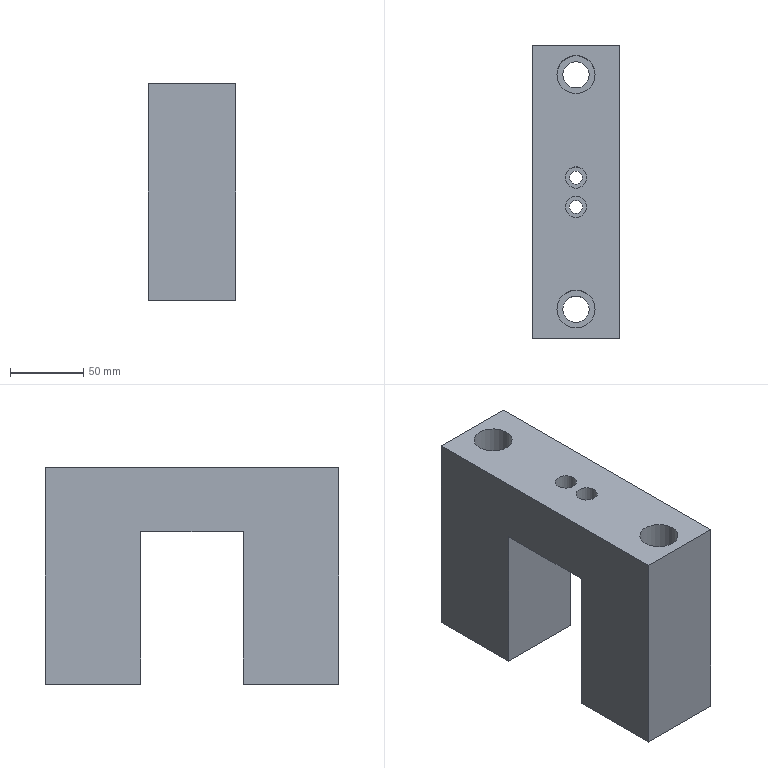Part | STEP file | lll_id2322_x_t | 1 solid | 22 faces | box 60 x 200 x 147.5 mm | volume 1187267 mm3 | plane 14 | cylinder 8 | commonest cylinder face diameters 9.009 x2 14.508 x2 18.009 x2 26.008 x2
STEP:
#1=CARTESIAN_POINT('',(3082.495,10.,341.5));
#2=VERTEX_POINT('',#1);
#3=CARTESIAN_POINT('',(3087.,10.,341.5));
#4=DIRECTION('',(0.,0.,-1.));
#5=DIRECTION('',(-1.,0.,0.));
#6=AXIS2_PLACEMENT_3D('',#3,#4,#5);
#7=CIRCLE('',#6,4.505);
#8=EDGE_CURVE('',#2,#2,#7,.T.);
#9=ORIENTED_EDGE('',*,*,#8,.F.);
#10=EDGE_LOOP('',(#9));
#11=FACE_BOUND('',#10,.T.);
#12=CARTESIAN_POINT('',(3091.505,10.,326.5));
#13=VERTEX_POINT('',#12);
#14=CARTESIAN_POINT('',(3087.,10.,326.5));
#15=DIRECTION('',(0.,0.,1.));
#16=DIRECTION('',(1.,0.,0.));
#17=AXIS2_PLACEMENT_3D('',#14,#15,#16);
#18=CIRCLE('',#17,4.505);
#19=EDGE_CURVE('',#13,#13,#18,.T.);
#20=ORIENTED_EDGE('',*,*,#19,.F.);
#21=EDGE_LOOP('',(#20));
#22=FACE_BOUND('',#21,.T.);
#23=CARTESIAN_POINT('',(3087.,10.,370.));
#24=DIRECTION('',(0.,0.,-1.));
#25=DIRECTION('',(1.,0.,0.));
#26=AXIS2_PLACEMENT_3D('',#23,#24,#25);
#27=CYLINDRICAL_SURFACE('',#26,4.505);
#28=ADVANCED_FACE('',(#11,#22),#27,.F.);
#29=CARTESIAN_POINT('',(3082.495,-10.,341.5));
#30=VERTEX_POINT('',#29);
#31=CARTESIAN_POINT('',(3087.,-10.,341.5));
#32=DIRECTION('',(0.,0.,-1.));
#33=DIRECTION('',(-1.,0.,0.));
#34=AXIS2_PLACEMENT_3D('',#31,#32,#33);
#35=CIRCLE('',#34,4.505);
#36=EDGE_CURVE('',#30,#30,#35,.T.);
#37=ORIENTED_EDGE('',*,*,#36,.F.);
#38=EDGE_LOOP('',(#37));
#39=FACE_BOUND('',#38,.T.);
#40=CARTESIAN_POINT('',(3091.505,-10.,326.5));
#41=VERTEX_POINT('',#40);
#42=CARTESIAN_POINT('',(3087.,-10.,326.5));
#43=DIRECTION('',(0.,0.,1.));
#44=DIRECTION('',(1.,0.,0.));
#45=AXIS2_PLACEMENT_3D('',#42,#43,#44);
#46=CIRCLE('',#45,4.505);
#47=EDGE_CURVE('',#41,#41,#46,.T.);
#48=ORIENTED_EDGE('',*,*,#47,.F.);
#49=EDGE_LOOP('',(#48));
#50=FACE_BOUND('',#49,.T.);
#51=CARTESIAN_POINT('',(3087.,-10.,370.));
#52=DIRECTION('',(0.,0.,-1.));
#53=DIRECTION('',(1.,0.,0.));
#54=AXIS2_PLACEMENT_3D('',#51,#52,#53);
#55=CYLINDRICAL_SURFACE('',#54,4.505);
#56=ADVANCED_FACE('',(#39,#50),#55,.F.);
#57=ORIENTED_EDGE('',*,*,#8,.T.);
#58=EDGE_LOOP('',(#57));
#59=FACE_BOUND('',#58,.T.);
#60=CARTESIAN_POINT('',(3094.254,10.,341.5));
#61=VERTEX_POINT('',#60);
#62=CARTESIAN_POINT('',(3087.,10.,341.5));
#63=DIRECTION('',(0.,0.,-1.));
#64=DIRECTION('',(1.,0.,0.));
#65=AXIS2_PLACEMENT_3D('',#62,#63,#64);
#66=CIRCLE('',#65,7.254);
#67=EDGE_CURVE('',#61,#61,#66,.T.);
#68=ORIENTED_EDGE('',*,*,#67,.F.);
#69=EDGE_LOOP('',(#68));
#70=FACE_BOUND('',#69,.T.);
#71=CARTESIAN_POINT('',(3087.,10.,341.5));
#72=DIRECTION('',(0.,0.,-1.));
#73=DIRECTION('',(-1.,0.,0.));
#74=AXIS2_PLACEMENT_3D('',#71,#72,#73);
#75=PLANE('',#74);
#76=ADVANCED_FACE('',(#59,#70),#75,.F.);
#77=ORIENTED_EDGE('',*,*,#36,.T.);
#78=EDGE_LOOP('',(#77));
#79=FACE_BOUND('',#78,.T.);
#80=CARTESIAN_POINT('',(3094.254,-10.,341.5));
#81=VERTEX_POINT('',#80);
#82=CARTESIAN_POINT('',(3087.,-10.,341.5));
#83=DIRECTION('',(0.,0.,-1.));
#84=DIRECTION('',(1.,0.,0.));
#85=AXIS2_PLACEMENT_3D('',#82,#83,#84);
#86=CIRCLE('',#85,7.254);
#87=EDGE_CURVE('',#81,#81,#86,.T.);
#88=ORIENTED_EDGE('',*,*,#87,.F.);
#89=EDGE_LOOP('',(#88));
#90=FACE_BOUND('',#89,.T.);
#91=CARTESIAN_POINT('',(3087.,-10.,341.5));
#92=DIRECTION('',(0.,0.,-1.));
#93=DIRECTION('',(-1.,0.,0.));
#94=AXIS2_PLACEMENT_3D('',#91,#92,#93);
#95=PLANE('',#94);
#96=ADVANCED_FACE('',(#79,#90),#95,.F.);
#97=CARTESIAN_POINT('',(3077.995,80.249,222.5));
#98=VERTEX_POINT('',#97);
#99=CARTESIAN_POINT('',(3087.,80.249,222.5));
#100=DIRECTION('',(0.,0.,-1.));
#101=DIRECTION('',(-1.,0.,0.));
#102=AXIS2_PLACEMENT_3D('',#99,#100,#101);
#103=CIRCLE('',#102,9.005);
#104=EDGE_CURVE('',#98,#98,#103,.T.);
#105=ORIENTED_EDGE('',*,*,#104,.F.);
#106=EDGE_LOOP('',(#105));
#107=FACE_BOUND('',#106,.T.);
#108=CARTESIAN_POINT('',(3117.,100.249,222.5));
#109=VERTEX_POINT('',#108);
#110=CARTESIAN_POINT('',(3057.,100.249,222.5));
#111=VERTEX_POINT('',#110);
#112=CARTESIAN_POINT('',(870.685,100.249,222.5));
#113=DIRECTION('',(-1.,0.,0.));
#114=VECTOR('',#113,1.);
#115=LINE('',#112,#114);
#116=EDGE_CURVE('',#109,#111,#115,.T.);
#117=ORIENTED_EDGE('',*,*,#116,.F.);
#118=CARTESIAN_POINT('',(3117.,35.249,222.5));
#119=VERTEX_POINT('',#118);
#120=CARTESIAN_POINT('',(3117.,-349.,222.5));
#121=DIRECTION('',(0.,-1.,0.));
#122=VECTOR('',#121,1.);
#123=LINE('',#120,#122);
#124=EDGE_CURVE('',#109,#119,#123,.T.);
#125=ORIENTED_EDGE('',*,*,#124,.T.);
#126=CARTESIAN_POINT('',(3057.,35.249,222.5));
#127=VERTEX_POINT('',#126);
#128=CARTESIAN_POINT('',(870.685,35.249,222.5));
#129=DIRECTION('',(1.,0.,0.));
#130=VECTOR('',#129,1.);
#131=LINE('',#128,#130);
#132=EDGE_CURVE('',#127,#119,#131,.T.);
#133=ORIENTED_EDGE('',*,*,#132,.F.);
#134=CARTESIAN_POINT('',(3057.,250.,222.5));
#135=DIRECTION('',(0.,-1.,0.));
#136=VECTOR('',#135,1.);
#137=LINE('',#134,#136);
#138=EDGE_CURVE('',#111,#127,#137,.T.);
#139=ORIENTED_EDGE('',*,*,#138,.F.);
#140=EDGE_LOOP('',(#117,#125,#133,#139));
#141=FACE_BOUND('',#140,.T.);
#142=CARTESIAN_POINT('',(870.685,-349.,222.5));
#143=DIRECTION('',(0.,0.,-1.));
#144=DIRECTION('',(1.,0.,0.));
#145=AXIS2_PLACEMENT_3D('',#142,#143,#144);
#146=PLANE('',#145);
#147=ADVANCED_FACE('',(#107,#141),#146,.T.);
#148=CARTESIAN_POINT('',(3057.,35.249,326.5));
#149=VERTEX_POINT('',#148);
#150=CARTESIAN_POINT('',(3057.,35.249,310.));
#151=DIRECTION('',(0.,0.,-1.));
#152=VECTOR('',#151,1.);
#153=LINE('',#150,#152);
#154=EDGE_CURVE('',#149,#127,#153,.T.);
#155=ORIENTED_EDGE('',*,*,#154,.T.);
#156=ORIENTED_EDGE('',*,*,#132,.T.);
#157=CARTESIAN_POINT('',(3117.,35.249,326.5));
#158=VERTEX_POINT('',#157);
#159=CARTESIAN_POINT('',(3117.,35.249,241.25));
#160=DIRECTION('',(0.,0.,-1.));
#161=VECTOR('',#160,1.);
#162=LINE('',#159,#161);
#163=EDGE_CURVE('',#158,#119,#162,.T.);
#164=ORIENTED_EDGE('',*,*,#163,.F.);
#165=CARTESIAN_POINT('',(3087.,35.249,326.5));
#166=DIRECTION('',(-1.,0.,0.));
#167=VECTOR('',#166,1.);
#168=LINE('',#165,#167);
#169=EDGE_CURVE('',#158,#149,#168,.T.);
#170=ORIENTED_EDGE('',*,*,#169,.T.);
#171=EDGE_LOOP('',(#155,#156,#164,#170));
#172=FACE_OUTER_BOUND('',#171,.T.);
#173=CARTESIAN_POINT('',(3087.,35.249,76.5));
#174=DIRECTION('',(0.,1.,0.));
#175=DIRECTION('',(0.,0.,1.));
#176=AXIS2_PLACEMENT_3D('',#173,#174,#175);
#177=PLANE('',#176);
#178=ADVANCED_FACE('',(#172),#177,.F.);
#179=ORIENTED_EDGE('',*,*,#47,.T.);
#180=EDGE_LOOP('',(#179));
#181=FACE_BOUND('',#180,.T.);
#182=ORIENTED_EDGE('',*,*,#19,.T.);
#183=EDGE_LOOP('',(#182));
#184=FACE_BOUND('',#183,.T.);
#185=CARTESIAN_POINT('',(3057.,-34.751,326.5));
#186=VERTEX_POINT('',#185);
#187=CARTESIAN_POINT('',(3057.,250.,326.5));
#188=DIRECTION('',(0.,1.,0.));
#189=VECTOR('',#188,1.);
#190=LINE('',#187,#189);
#191=EDGE_CURVE('',#186,#149,#190,.T.);
#192=ORIENTED_EDGE('',*,*,#191,.T.);
#193=ORIENTED_EDGE('',*,*,#169,.F.);
#194=CARTESIAN_POINT('',(3117.,-34.751,326.5));
#195=VERTEX_POINT('',#194);
#196=CARTESIAN_POINT('',(3117.,-350.,326.5));
#197=DIRECTION('',(0.,1.,0.));
#198=VECTOR('',#197,1.);
#199=LINE('',#196,#198);
#200=EDGE_CURVE('',#195,#158,#199,.T.);
#201=ORIENTED_EDGE('',*,*,#200,.F.);
#202=CARTESIAN_POINT('',(3087.,-34.751,326.5));
#203=DIRECTION('',(1.,0.,0.));
#204=VECTOR('',#203,1.);
#205=LINE('',#202,#204);
#206=EDGE_CURVE('',#186,#195,#205,.T.);
#207=ORIENTED_EDGE('',*,*,#206,.F.);
#208=EDGE_LOOP('',(#192,#193,#201,#207));
#209=FACE_BOUND('',#208,.T.);
#210=CARTESIAN_POINT('',(3087.,0.2492,326.5));
#211=DIRECTION('',(0.,0.,1.));
#212=DIRECTION('',(1.,0.,0.));
#213=AXIS2_PLACEMENT_3D('',#210,#211,#212);
#214=PLANE('',#213);
#215=ADVANCED_FACE('',(#181,#184,#209),#214,.F.);
#216=CARTESIAN_POINT('',(3057.,-34.751,222.5));
#217=VERTEX_POINT('',#216);
#218=CARTESIAN_POINT('',(3057.,-34.751,310.));
#219=DIRECTION('',(0.,0.,1.));
#220=VECTOR('',#219,1.);
#221=LINE('',#218,#220);
#222=EDGE_CURVE('',#217,#186,#221,.T.);
#223=ORIENTED_EDGE('',*,*,#222,.T.);
#224=ORIENTED_EDGE('',*,*,#206,.T.);
#225=CARTESIAN_POINT('',(3117.,-34.751,222.5));
#226=VERTEX_POINT('',#225);
#227=CARTESIAN_POINT('',(3117.,-34.751,241.25));
#228=DIRECTION('',(0.,0.,1.));
#229=VECTOR('',#228,1.);
#230=LINE('',#227,#229);
#231=EDGE_CURVE('',#226,#195,#230,.T.);
#232=ORIENTED_EDGE('',*,*,#231,.F.);
#233=CARTESIAN_POINT('',(870.685,-34.751,222.5));
#234=DIRECTION('',(-1.,0.,0.));
#235=VECTOR('',#234,1.);
#236=LINE('',#233,#235);
#237=EDGE_CURVE('',#226,#217,#236,.T.);
#238=ORIENTED_EDGE('',*,*,#237,.T.);
#239=EDGE_LOOP('',(#223,#224,#232,#238));
#240=FACE_OUTER_BOUND('',#239,.T.);
#241=CARTESIAN_POINT('',(3087.,-34.751,76.5));
#242=DIRECTION('',(0.,-1.,0.));
#243=DIRECTION('',(0.,0.,-1.));
#244=AXIS2_PLACEMENT_3D('',#241,#242,#243);
#245=PLANE('',#244);
#246=ADVANCED_FACE('',(#240),#245,.F.);
#247=CARTESIAN_POINT('',(3057.,100.249,370.));
#248=VERTEX_POINT('',#247);
#249=CARTESIAN_POINT('',(3057.,100.249,310.));
#250=DIRECTION('',(0.,0.,-1.));
#251=VECTOR('',#250,1.);
#252=LINE('',#249,#251);
#253=EDGE_CURVE('',#248,#111,#252,.T.);
#254=ORIENTED_EDGE('',*,*,#253,.F.);
#255=CARTESIAN_POINT('',(3117.,100.249,370.));
#256=VERTEX_POINT('',#255);
#257=CARTESIAN_POINT('',(870.685,100.249,370.));
#258=DIRECTION('',(1.,0.,0.));
#259=VECTOR('',#258,1.);
#260=LINE('',#257,#259);
#261=EDGE_CURVE('',#248,#256,#260,.T.);
#262=ORIENTED_EDGE('',*,*,#261,.T.);
#263=CARTESIAN_POINT('',(3117.,100.249,241.25));
#264=DIRECTION('',(0.,0.,-1.));
#265=VECTOR('',#264,1.);
#266=LINE('',#263,#265);
#267=EDGE_CURVE('',#256,#109,#266,.T.);
#268=ORIENTED_EDGE('',*,*,#267,.T.);
#269=ORIENTED_EDGE('',*,*,#116,.T.);
#270=EDGE_LOOP('',(#254,#262,#268,#269));
#271=FACE_OUTER_BOUND('',#270,.T.);
#272=CARTESIAN_POINT('',(3087.,100.249,224.5));
#273=DIRECTION('',(0.,-1.,0.));
#274=DIRECTION('',(0.,0.,-1.));
#275=AXIS2_PLACEMENT_3D('',#272,#273,#274);
#276=PLANE('',#275);
#277=ADVANCED_FACE('',(#271),#276,.F.);
#278=ORIENTED_EDGE('',*,*,#67,.T.);
#279=EDGE_LOOP('',(#278));
#280=FACE_BOUND('',#279,.T.);
#281=CARTESIAN_POINT('',(3094.254,10.,370.));
#282=VERTEX_POINT('',#281);
#283=CARTESIAN_POINT('',(3087.,10.,370.));
#284=DIRECTION('',(0.,0.,-1.));
#285=DIRECTION('',(1.,0.,0.));
#286=AXIS2_PLACEMENT_3D('',#283,#284,#285);
#287=CIRCLE('',#286,7.254);
#288=EDGE_CURVE('',#282,#282,#287,.T.);
#289=ORIENTED_EDGE('',*,*,#288,.F.);
#290=EDGE_LOOP('',(#289));
#291=FACE_BOUND('',#290,.T.);
#292=CARTESIAN_POINT('',(3087.,10.,370.));
#293=DIRECTION('',(0.,0.,-1.));
#294=DIRECTION('',(1.,0.,0.));
#295=AXIS2_PLACEMENT_3D('',#292,#293,#294);
#296=CYLINDRICAL_SURFACE('',#295,7.254);
#297=ADVANCED_FACE('',(#280,#291),#296,.F.);
#298=ORIENTED_EDGE('',*,*,#87,.T.);
#299=EDGE_LOOP('',(#298));
#300=FACE_BOUND('',#299,.T.);
#301=CARTESIAN_POINT('',(3094.254,-10.,370.));
#302=VERTEX_POINT('',#301);
#303=CARTESIAN_POINT('',(3087.,-10.,370.));
#304=DIRECTION('',(0.,0.,-1.));
#305=DIRECTION('',(1.,0.,0.));
#306=AXIS2_PLACEMENT_3D('',#303,#304,#305);
#307=CIRCLE('',#306,7.254);
#308=EDGE_CURVE('',#302,#302,#307,.T.);
#309=ORIENTED_EDGE('',*,*,#308,.F.);
#310=EDGE_LOOP('',(#309));
#311=FACE_BOUND('',#310,.T.);
#312=CARTESIAN_POINT('',(3087.,-10.,370.));
#313=DIRECTION('',(0.,0.,-1.));
#314=DIRECTION('',(1.,0.,0.));
#315=AXIS2_PLACEMENT_3D('',#312,#313,#314);
#316=CYLINDRICAL_SURFACE('',#315,7.254);
#317=ADVANCED_FACE('',(#300,#311),#316,.F.);
#318=CARTESIAN_POINT('',(3100.004,-79.751,370.));
#319=VERTEX_POINT('',#318);
#320=CARTESIAN_POINT('',(3087.,-79.751,370.));
#321=DIRECTION('',(0.,0.,-1.));
#322=DIRECTION('',(1.,0.,0.));
#323=AXIS2_PLACEMENT_3D('',#320,#321,#322);
#324=CIRCLE('',#323,13.004);
#325=EDGE_CURVE('',#319,#319,#324,.T.);
#326=ORIENTED_EDGE('',*,*,#325,.T.);
#327=EDGE_LOOP('',(#326));
#328=FACE_BOUND('',#327,.T.);
#329=CARTESIAN_POINT('',(3100.004,80.249,370.));
#330=VERTEX_POINT('',#329);
#331=CARTESIAN_POINT('',(3087.,80.249,370.));
#332=DIRECTION('',(0.,0.,-1.));
#333=DIRECTION('',(1.,0.,0.));
#334=AXIS2_PLACEMENT_3D('',#331,#332,#333);
#335=CIRCLE('',#334,13.004);
#336=EDGE_CURVE('',#330,#330,#335,.T.);
#337=ORIENTED_EDGE('',*,*,#336,.T.);
#338=EDGE_LOOP('',(#337));
#339=FACE_BOUND('',#338,.T.);
#340=ORIENTED_EDGE('',*,*,#308,.T.);
#341=EDGE_LOOP('',(#340));
#342=FACE_BOUND('',#341,.T.);
#343=ORIENTED_EDGE('',*,*,#288,.T.);
#344=EDGE_LOOP('',(#343));
#345=FACE_BOUND('',#344,.T.);
#346=CARTESIAN_POINT('',(3057.,-99.751,370.));
#347=VERTEX_POINT('',#346);
#348=CARTESIAN_POINT('',(3057.,250.,370.));
#349=DIRECTION('',(0.,-1.,0.));
#350=VECTOR('',#349,1.);
#351=LINE('',#348,#350);
#352=EDGE_CURVE('',#248,#347,#351,.T.);
#353=ORIENTED_EDGE('',*,*,#352,.T.);
#354=CARTESIAN_POINT('',(3117.,-99.751,370.));
#355=VERTEX_POINT('',#354);
#356=CARTESIAN_POINT('',(870.685,-99.751,370.));
#357=DIRECTION('',(-1.,0.,0.));
#358=VECTOR('',#357,1.);
#359=LINE('',#356,#358);
#360=EDGE_CURVE('',#355,#347,#359,.T.);
#361=ORIENTED_EDGE('',*,*,#360,.F.);
#362=CARTESIAN_POINT('',(3117.,-349.,370.));
#363=DIRECTION('',(0.,1.,0.));
#364=VECTOR('',#363,1.);
#365=LINE('',#362,#364);
#366=EDGE_CURVE('',#355,#256,#365,.T.);
#367=ORIENTED_EDGE('',*,*,#366,.T.);
#368=ORIENTED_EDGE('',*,*,#261,.F.);
#369=EDGE_LOOP('',(#353,#361,#367,#368));
#370=FACE_BOUND('',#369,.T.);
#371=CARTESIAN_POINT('',(870.685,-349.,370.));
#372=DIRECTION('',(0.,0.,-1.));
#373=DIRECTION('',(1.,0.,0.));
#374=AXIS2_PLACEMENT_3D('',#371,#372,#373);
#375=PLANE('',#374);
#376=ADVANCED_FACE('',(#328,#339,#342,#345,#370),#375,.F.);
#377=ORIENTED_EDGE('',*,*,#366,.F.);
#378=CARTESIAN_POINT('',(3117.,-99.751,222.5));
#379=VERTEX_POINT('',#378);
#380=CARTESIAN_POINT('',(3117.,-99.751,241.25));
#381=DIRECTION('',(0.,0.,1.));
#382=VECTOR('',#381,1.);
#383=LINE('',#380,#382);
#384=EDGE_CURVE('',#379,#355,#383,.T.);
#385=ORIENTED_EDGE('',*,*,#384,.F.);
#386=CARTESIAN_POINT('',(3117.,-349.,222.5));
#387=DIRECTION('',(0.,-1.,0.));
#388=VECTOR('',#387,1.);
#389=LINE('',#386,#388);
#390=EDGE_CURVE('',#226,#379,#389,.T.);
#391=ORIENTED_EDGE('',*,*,#390,.F.);
#392=ORIENTED_EDGE('',*,*,#231,.T.);
#393=ORIENTED_EDGE('',*,*,#200,.T.);
#394=ORIENTED_EDGE('',*,*,#163,.T.);
#395=ORIENTED_EDGE('',*,*,#124,.F.);
#396=ORIENTED_EDGE('',*,*,#267,.F.);
#397=EDGE_LOOP('',(#377,#385,#391,#392,#393,#394,#395,#396));
#398=FACE_OUTER_BOUND('',#397,.T.);
#399=CARTESIAN_POINT('',(3117.,-350.,241.25));
#400=DIRECTION('',(-1.,0.,0.));
#401=DIRECTION('',(0.,0.,-1.));
#402=AXIS2_PLACEMENT_3D('',#399,#400,#401);
#403=PLANE('',#402);
#404=ADVANCED_FACE('',(#398),#403,.F.);
#405=CARTESIAN_POINT('',(3057.,-99.751,222.5));
#406=VERTEX_POINT('',#405);
#407=CARTESIAN_POINT('',(3057.,-99.751,310.));
#408=DIRECTION('',(0.,0.,1.));
#409=VECTOR('',#408,1.);
#410=LINE('',#407,#409);
#411=EDGE_CURVE('',#406,#347,#410,.T.);
#412=ORIENTED_EDGE('',*,*,#411,.T.);
#413=ORIENTED_EDGE('',*,*,#352,.F.);
#414=ORIENTED_EDGE('',*,*,#253,.T.);
#415=ORIENTED_EDGE('',*,*,#138,.T.);
#416=ORIENTED_EDGE('',*,*,#154,.F.);
#417=ORIENTED_EDGE('',*,*,#191,.F.);
#418=ORIENTED_EDGE('',*,*,#222,.F.);
#419=CARTESIAN_POINT('',(3057.,250.,222.5));
#420=DIRECTION('',(0.,-1.,0.));
#421=VECTOR('',#420,1.);
#422=LINE('',#419,#421);
#423=EDGE_CURVE('',#217,#406,#422,.T.);
#424=ORIENTED_EDGE('',*,*,#423,.T.);
#425=EDGE_LOOP('',(#412,#413,#414,#415,#416,#417,#418,#424));
#426=FACE_OUTER_BOUND('',#425,.T.);
#427=CARTESIAN_POINT('',(3057.,250.,310.));
#428=DIRECTION('',(-1.,0.,0.));
#429=DIRECTION('',(0.,0.,-1.));
#430=AXIS2_PLACEMENT_3D('',#427,#428,#429);
#431=PLANE('',#430);
#432=ADVANCED_FACE('',(#426),#431,.T.);
#433=CARTESIAN_POINT('',(3077.995,-79.751,222.5));
#434=VERTEX_POINT('',#433);
#435=CARTESIAN_POINT('',(3087.,-79.751,222.5));
#436=DIRECTION('',(0.,0.,-1.));
#437=DIRECTION('',(-1.,0.,0.));
#438=AXIS2_PLACEMENT_3D('',#435,#436,#437);
#439=CIRCLE('',#438,9.005);
#440=EDGE_CURVE('',#434,#434,#439,.T.);
#441=ORIENTED_EDGE('',*,*,#440,.F.);
#442=EDGE_LOOP('',(#441));
#443=FACE_BOUND('',#442,.T.);
#444=CARTESIAN_POINT('',(870.685,-99.751,222.5));
#445=DIRECTION('',(-1.,0.,0.));
#446=VECTOR('',#445,1.);
#447=LINE('',#444,#446);
#448=EDGE_CURVE('',#379,#406,#447,.T.);
#449=ORIENTED_EDGE('',*,*,#448,.T.);
#450=ORIENTED_EDGE('',*,*,#423,.F.);
#451=ORIENTED_EDGE('',*,*,#237,.F.);
#452=ORIENTED_EDGE('',*,*,#390,.T.);
#453=EDGE_LOOP('',(#449,#450,#451,#452));
#454=FACE_BOUND('',#453,.T.);
#455=CARTESIAN_POINT('',(870.685,-349.,222.5));
#456=DIRECTION('',(0.,0.,-1.));
#457=DIRECTION('',(1.,0.,0.));
#458=AXIS2_PLACEMENT_3D('',#455,#456,#457);
#459=PLANE('',#458);
#460=ADVANCED_FACE('',(#443,#454),#459,.T.);
#461=ORIENTED_EDGE('',*,*,#448,.F.);
#462=ORIENTED_EDGE('',*,*,#384,.T.);
#463=ORIENTED_EDGE('',*,*,#360,.T.);
#464=ORIENTED_EDGE('',*,*,#411,.F.);
#465=EDGE_LOOP('',(#461,#462,#463,#464));
#466=FACE_OUTER_BOUND('',#465,.T.);
#467=CARTESIAN_POINT('',(3087.,-99.751,224.5));
#468=DIRECTION('',(0.,1.,0.));
#469=DIRECTION('',(0.,0.,1.));
#470=AXIS2_PLACEMENT_3D('',#467,#468,#469);
#471=PLANE('',#470);
#472=ADVANCED_FACE('',(#466),#471,.F.);
#473=ORIENTED_EDGE('',*,*,#104,.T.);
#474=EDGE_LOOP('',(#473));
#475=FACE_BOUND('',#474,.T.);
#476=CARTESIAN_POINT('',(3077.995,80.249,262.5));
#477=VERTEX_POINT('',#476);
#478=CARTESIAN_POINT('',(3087.,80.249,262.5));
#479=DIRECTION('',(0.,0.,-1.));
#480=DIRECTION('',(-1.,0.,0.));
#481=AXIS2_PLACEMENT_3D('',#478,#479,#480);
#482=CIRCLE('',#481,9.005);
#483=EDGE_CURVE('',#477,#477,#482,.T.);
#484=ORIENTED_EDGE('',*,*,#483,.F.);
#485=EDGE_LOOP('',(#484));
#486=FACE_BOUND('',#485,.T.);
#487=CARTESIAN_POINT('',(3087.,80.249,422.));
#488=DIRECTION('',(0.,0.,-1.));
#489=DIRECTION('',(1.,0.,0.));
#490=AXIS2_PLACEMENT_3D('',#487,#488,#489);
#491=CYLINDRICAL_SURFACE('',#490,9.005);
#492=ADVANCED_FACE('',(#475,#486),#491,.F.);
#493=ORIENTED_EDGE('',*,*,#483,.T.);
#494=EDGE_LOOP('',(#493));
#495=FACE_BOUND('',#494,.T.);
#496=CARTESIAN_POINT('',(3100.004,80.249,262.5));
#497=VERTEX_POINT('',#496);
#498=CARTESIAN_POINT('',(3087.,80.249,262.5));
#499=DIRECTION('',(0.,0.,-1.));
#500=DIRECTION('',(1.,0.,0.));
#501=AXIS2_PLACEMENT_3D('',#498,#499,#500);
#502=CIRCLE('',#501,13.004);
#503=EDGE_CURVE('',#497,#497,#502,.T.);
#504=ORIENTED_EDGE('',*,*,#503,.F.);
#505=EDGE_LOOP('',(#504));
#506=FACE_BOUND('',#505,.T.);
#507=CARTESIAN_POINT('',(3087.,80.249,262.5));
#508=DIRECTION('',(0.,0.,-1.));
#509=DIRECTION('',(-1.,0.,0.));
#510=AXIS2_PLACEMENT_3D('',#507,#508,#509);
#511=PLANE('',#510);
#512=ADVANCED_FACE('',(#495,#506),#511,.F.);
#513=ORIENTED_EDGE('',*,*,#503,.T.);
#514=EDGE_LOOP('',(#513));
#515=FACE_BOUND('',#514,.T.);
#516=ORIENTED_EDGE('',*,*,#336,.F.);
#517=EDGE_LOOP('',(#516));
#518=FACE_BOUND('',#517,.T.);
#519=CARTESIAN_POINT('',(3087.,80.249,370.));
#520=DIRECTION('',(0.,0.,-1.));
#521=DIRECTION('',(1.,0.,0.));
#522=AXIS2_PLACEMENT_3D('',#519,#520,#521);
#523=CYLINDRICAL_SURFACE('',#522,13.004);
#524=ADVANCED_FACE('',(#515,#518),#523,.F.);
#525=ORIENTED_EDGE('',*,*,#440,.T.);
#526=EDGE_LOOP('',(#525));
#527=FACE_BOUND('',#526,.T.);
#528=CARTESIAN_POINT('',(3077.995,-79.751,262.5));
#529=VERTEX_POINT('',#528);
#530=CARTESIAN_POINT('',(3087.,-79.751,262.5));
#531=DIRECTION('',(0.,0.,-1.));
#532=DIRECTION('',(-1.,0.,0.));
#533=AXIS2_PLACEMENT_3D('',#530,#531,#532);
#534=CIRCLE('',#533,9.005);
#535=EDGE_CURVE('',#529,#529,#534,.T.);
#536=ORIENTED_EDGE('',*,*,#535,.F.);
#537=EDGE_LOOP('',(#536));
#538=FACE_BOUND('',#537,.T.);
#539=CARTESIAN_POINT('',(3087.,-79.751,422.));
#540=DIRECTION('',(0.,0.,-1.));
#541=DIRECTION('',(1.,0.,0.));
#542=AXIS2_PLACEMENT_3D('',#539,#540,#541);
#543=CYLINDRICAL_SURFACE('',#542,9.005);
#544=ADVANCED_FACE('',(#527,#538),#543,.F.);
#545=ORIENTED_EDGE('',*,*,#535,.T.);
#546=EDGE_LOOP('',(#545));
#547=FACE_BOUND('',#546,.T.);
#548=CARTESIAN_POINT('',(3100.004,-79.751,262.5));
#549=VERTEX_POINT('',#548);
#550=CARTESIAN_POINT('',(3087.,-79.751,262.5));
#551=DIRECTION('',(0.,0.,-1.));
#552=DIRECTION('',(1.,0.,0.));
#553=AXIS2_PLACEMENT_3D('',#550,#551,#552);
#554=CIRCLE('',#553,13.004);
#555=EDGE_CURVE('',#549,#549,#554,.T.);
#556=ORIENTED_EDGE('',*,*,#555,.F.);
#557=EDGE_LOOP('',(#556));
#558=FACE_BOUND('',#557,.T.);
#559=CARTESIAN_POINT('',(3087.,-79.751,262.5));
#560=DIRECTION('',(0.,0.,-1.));
#561=DIRECTION('',(-1.,0.,0.));
#562=AXIS2_PLACEMENT_3D('',#559,#560,#561);
#563=PLANE('',#562);
#564=ADVANCED_FACE('',(#547,#558),#563,.F.);
#565=ORIENTED_EDGE('',*,*,#555,.T.);
#566=EDGE_LOOP('',(#565));
#567=FACE_BOUND('',#566,.T.);
#568=ORIENTED_EDGE('',*,*,#325,.F.);
#569=EDGE_LOOP('',(#568));
#570=FACE_BOUND('',#569,.T.);
#571=CARTESIAN_POINT('',(3087.,-79.751,370.));
#572=DIRECTION('',(0.,0.,-1.));
#573=DIRECTION('',(1.,0.,0.));
#574=AXIS2_PLACEMENT_3D('',#571,#572,#573);
#575=CYLINDRICAL_SURFACE('',#574,13.004);
#576=ADVANCED_FACE('',(#567,#570),#575,.F.);
#577=CLOSED_SHELL('',(#28,#56,#76,#96,#147,#178,#215,#246,#277,#297,#317,#376,#404,#432,#460,#472,#492,#512,#524,#544,#564,#576));
#578=MANIFOLD_SOLID_BREP('',#577);
#579=(LENGTH_UNIT()NAMED_UNIT(*)SI_UNIT(.MILLI.,.METRE.));
#580=UNCERTAINTY_MEASURE_WITH_UNIT(LENGTH_MEASURE(0.00002),#579,'','');
#581=(NAMED_UNIT(*)PLANE_ANGLE_UNIT()SI_UNIT($,.RADIAN.));
#582=PLANE_ANGLE_MEASURE_WITH_UNIT(PLANE_ANGLE_MEASURE(0.01745),#581);
#583=DIMENSIONAL_EXPONENTS(0.,0.,0.,0.,0.,0.,0.);
#584=(CONVERSION_BASED_UNIT('DEGREE',#582)NAMED_UNIT(#583)PLANE_ANGLE_UNIT());
#585=(NAMED_UNIT(*)SI_UNIT($,.STERADIAN.)SOLID_ANGLE_UNIT());
#586=(GEOMETRIC_REPRESENTATION_CONTEXT(3)GLOBAL_UNCERTAINTY_ASSIGNED_CONTEXT((#580))GLOBAL_UNIT_ASSIGNED_CONTEXT((#579,#584,#585))REPRESENTATION_CONTEXT('',''));
#587=ADVANCED_BREP_SHAPE_REPRESENTATION('',(#578),#586);